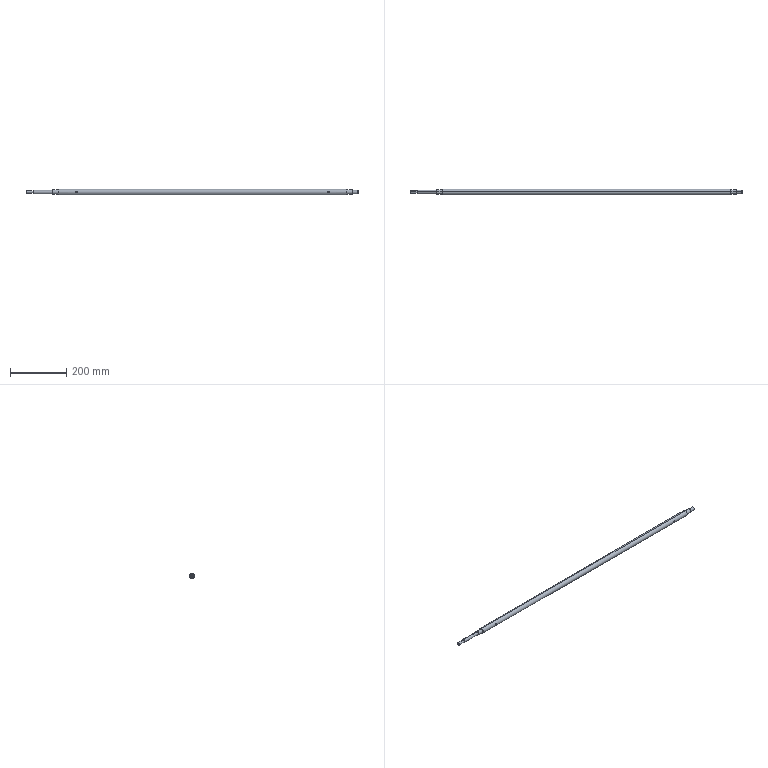Part | NX | features BREP 1 | 1 solid | 32 faces | box 1181 x 20 x 20 mm | volume 340275 mm3 | cylinder 18 | plane 10 | cone 4 | commonest cylinder face diameters 6 x4 12 x4 15 x4 4 x2 10 x2 20 x2
STEP:
#1=CARTESIAN_POINT('',(630.967,-9.539,-3.));
#2=VERTEX_POINT('',#1);
#3=CARTESIAN_POINT('',(630.967,-9.539,3.));
#4=VERTEX_POINT('',#3);
#5=CARTESIAN_POINT('',(630.967,-9.539,-3.));
#6=CARTESIAN_POINT('',(630.17,-9.539,-3.));
#7=CARTESIAN_POINT('',(628.623,-9.775,-2.35));
#8=CARTESIAN_POINT('',(627.639,-10.112,-0.004774));
#9=CARTESIAN_POINT('',(628.622,-9.775,2.351));
#10=CARTESIAN_POINT('',(630.17,-9.539,3.));
#11=CARTESIAN_POINT('',(630.967,-9.539,3.));
#12=B_SPLINE_CURVE_WITH_KNOTS('',3,(#5,#6,#7,#8,#9,#10,#11),.UNSPECIFIED.,.F.,.F.,(4,1,1,1,4),(0.,0.002358,0.004715,0.007073,0.009431),.UNSPECIFIED.);
#13=EDGE_CURVE('',#2,#4,#12,.T.);
#14=ORIENTED_EDGE('',*,*,#13,.F.);
#15=CARTESIAN_POINT('',(630.967,9.539,-3.));
#16=VERTEX_POINT('',#15);
#17=CARTESIAN_POINT('',(630.967,-10.,-3.));
#18=DIRECTION('',(0.,1.,0.));
#19=VECTOR('',#18,1000.);
#20=LINE('',#17,#19);
#21=EDGE_CURVE('',#2,#16,#20,.T.);
#22=ORIENTED_EDGE('',*,*,#21,.T.);
#23=CARTESIAN_POINT('',(630.967,9.539,3.));
#24=VERTEX_POINT('',#23);
#25=CARTESIAN_POINT('',(630.967,9.539,3.));
#26=CARTESIAN_POINT('',(630.17,9.539,3.));
#27=CARTESIAN_POINT('',(628.623,9.775,2.35));
#28=CARTESIAN_POINT('',(627.639,10.112,0.004774));
#29=CARTESIAN_POINT('',(628.622,9.775,-2.351));
#30=CARTESIAN_POINT('',(630.17,9.539,-3.));
#31=CARTESIAN_POINT('',(630.967,9.539,-3.));
#32=B_SPLINE_CURVE_WITH_KNOTS('',3,(#25,#26,#27,#28,#29,#30,#31),.UNSPECIFIED.,.F.,.F.,(4,1,1,1,4),(0.,0.002358,0.004715,0.007073,0.009431),.UNSPECIFIED.);
#33=EDGE_CURVE('',#24,#16,#32,.T.);
#34=ORIENTED_EDGE('',*,*,#33,.F.);
#35=CARTESIAN_POINT('',(630.967,-10.,3.));
#36=DIRECTION('',(0.,1.,0.));
#37=VECTOR('',#36,1000.);
#38=LINE('',#35,#37);
#39=EDGE_CURVE('',#4,#24,#38,.T.);
#40=ORIENTED_EDGE('',*,*,#39,.F.);
#41=EDGE_LOOP('',(#14,#22,#34,#40));
#42=FACE_BOUND('',#41,.T.);
#43=CARTESIAN_POINT('',(630.967,-10.,0.));
#44=DIRECTION('',(0.,1.,0.));
#45=DIRECTION('',(0.,0.,-1.));
#46=AXIS2_PLACEMENT_3D('',#43,#44,#45);
#47=CYLINDRICAL_SURFACE('',#46,3.);
#48=ADVANCED_FACE('',(#42),#47,.F.);
#49=CARTESIAN_POINT('',(-265.033,-9.539,-3.));
#50=VERTEX_POINT('',#49);
#51=CARTESIAN_POINT('',(-265.033,-9.539,3.));
#52=VERTEX_POINT('',#51);
#53=CARTESIAN_POINT('',(-265.033,-9.539,-3.));
#54=CARTESIAN_POINT('',(-265.83,-9.539,-3.));
#55=CARTESIAN_POINT('',(-267.377,-9.775,-2.35));
#56=CARTESIAN_POINT('',(-268.361,-10.112,-0.004774));
#57=CARTESIAN_POINT('',(-267.378,-9.775,2.351));
#58=CARTESIAN_POINT('',(-265.83,-9.539,3.));
#59=CARTESIAN_POINT('',(-265.033,-9.539,3.));
#60=B_SPLINE_CURVE_WITH_KNOTS('',3,(#53,#54,#55,#56,#57,#58,#59),.UNSPECIFIED.,.F.,.F.,(4,1,1,1,4),(0.,0.002358,0.004715,0.007073,0.009431),.UNSPECIFIED.);
#61=EDGE_CURVE('',#50,#52,#60,.T.);
#62=ORIENTED_EDGE('',*,*,#61,.F.);
#63=CARTESIAN_POINT('',(-265.033,9.539,-3.));
#64=VERTEX_POINT('',#63);
#65=CARTESIAN_POINT('',(-265.033,-10.,-3.));
#66=DIRECTION('',(0.,1.,0.));
#67=VECTOR('',#66,1000.);
#68=LINE('',#65,#67);
#69=EDGE_CURVE('',#50,#64,#68,.T.);
#70=ORIENTED_EDGE('',*,*,#69,.T.);
#71=CARTESIAN_POINT('',(-265.033,9.539,3.));
#72=VERTEX_POINT('',#71);
#73=CARTESIAN_POINT('',(-265.033,9.539,3.));
#74=CARTESIAN_POINT('',(-265.83,9.539,3.));
#75=CARTESIAN_POINT('',(-267.377,9.775,2.35));
#76=CARTESIAN_POINT('',(-268.361,10.112,0.004774));
#77=CARTESIAN_POINT('',(-267.378,9.775,-2.351));
#78=CARTESIAN_POINT('',(-265.83,9.539,-3.));
#79=CARTESIAN_POINT('',(-265.033,9.539,-3.));
#80=B_SPLINE_CURVE_WITH_KNOTS('',3,(#73,#74,#75,#76,#77,#78,#79),.UNSPECIFIED.,.F.,.F.,(4,1,1,1,4),(0.,0.002358,0.004715,0.007073,0.009431),.UNSPECIFIED.);
#81=EDGE_CURVE('',#72,#64,#80,.T.);
#82=ORIENTED_EDGE('',*,*,#81,.F.);
#83=CARTESIAN_POINT('',(-265.033,-10.,3.));
#84=DIRECTION('',(0.,1.,0.));
#85=VECTOR('',#84,1000.);
#86=LINE('',#83,#85);
#87=EDGE_CURVE('',#52,#72,#86,.T.);
#88=ORIENTED_EDGE('',*,*,#87,.F.);
#89=EDGE_LOOP('',(#62,#70,#82,#88));
#90=FACE_BOUND('',#89,.T.);
#91=CARTESIAN_POINT('',(-265.033,-10.,0.));
#92=DIRECTION('',(0.,1.,0.));
#93=DIRECTION('',(0.,0.,-1.));
#94=AXIS2_PLACEMENT_3D('',#91,#92,#93);
#95=CYLINDRICAL_SURFACE('',#94,3.);
#96=ADVANCED_FACE('',(#90),#95,.F.);
#97=CARTESIAN_POINT('',(735.967,0.,5.));
#98=VERTEX_POINT('',#97);
#99=CARTESIAN_POINT('',(735.967,0.,-5.));
#100=VERTEX_POINT('',#99);
#101=CARTESIAN_POINT('',(735.967,0.,0.));
#102=DIRECTION('',(-1.,0.,0.));
#103=DIRECTION('',(0.,0.,1.));
#104=AXIS2_PLACEMENT_3D('',#101,#102,#103);
#105=CIRCLE('',#104,5.);
#106=EDGE_CURVE('',#98,#100,#105,.T.);
#107=ORIENTED_EDGE('',*,*,#106,.T.);
#108=CARTESIAN_POINT('',(734.967,0.,-6.));
#109=VERTEX_POINT('',#108);
#110=CARTESIAN_POINT('',(735.967,0.,-5.));
#111=DIRECTION('',(-0.7071,0.,-0.7071));
#112=VECTOR('',#111,1000.);
#113=LINE('',#110,#112);
#114=EDGE_CURVE('',#100,#109,#113,.T.);
#115=ORIENTED_EDGE('',*,*,#114,.T.);
#116=CARTESIAN_POINT('',(734.967,0.,6.));
#117=VERTEX_POINT('',#116);
#118=CARTESIAN_POINT('',(734.967,0.,0.));
#119=DIRECTION('',(-1.,0.,0.));
#120=DIRECTION('',(0.,0.,1.));
#121=AXIS2_PLACEMENT_3D('',#118,#119,#120);
#122=CIRCLE('',#121,6.);
#123=EDGE_CURVE('',#117,#109,#122,.T.);
#124=ORIENTED_EDGE('',*,*,#123,.F.);
#125=CARTESIAN_POINT('',(735.967,0.,5.));
#126=DIRECTION('',(-0.7071,0.,0.7071));
#127=VECTOR('',#126,1000.);
#128=LINE('',#125,#127);
#129=EDGE_CURVE('',#98,#117,#128,.T.);
#130=ORIENTED_EDGE('',*,*,#129,.F.);
#131=EDGE_LOOP('',(#107,#115,#124,#130));
#132=FACE_BOUND('',#131,.T.);
#133=CARTESIAN_POINT('',(735.967,0.,0.));
#134=DIRECTION('',(-1.,0.,0.));
#135=DIRECTION('',(0.,0.,-1.));
#136=AXIS2_PLACEMENT_3D('',#133,#134,#135);
#137=CONICAL_SURFACE('',#136,5.,0.7854);
#138=ADVANCED_FACE('',(#132),#137,.T.);
#139=ORIENTED_EDGE('',*,*,#123,.T.);
#140=CARTESIAN_POINT('',(715.967,0.,-6.));
#141=VERTEX_POINT('',#140);
#142=CARTESIAN_POINT('',(-445.033,0.,-6.));
#143=DIRECTION('',(-1.,0.,0.));
#144=VECTOR('',#143,1000.);
#145=LINE('',#142,#144);
#146=EDGE_CURVE('',#109,#141,#145,.T.);
#147=ORIENTED_EDGE('',*,*,#146,.T.);
#148=CARTESIAN_POINT('',(715.967,0.,6.));
#149=VERTEX_POINT('',#148);
#150=CARTESIAN_POINT('',(715.967,0.,0.));
#151=DIRECTION('',(-1.,0.,0.));
#152=DIRECTION('',(0.,0.,1.));
#153=AXIS2_PLACEMENT_3D('',#150,#151,#152);
#154=CIRCLE('',#153,6.);
#155=EDGE_CURVE('',#149,#141,#154,.T.);
#156=ORIENTED_EDGE('',*,*,#155,.F.);
#157=CARTESIAN_POINT('',(-445.033,0.,6.));
#158=DIRECTION('',(-1.,0.,0.));
#159=VECTOR('',#158,1000.);
#160=LINE('',#157,#159);
#161=EDGE_CURVE('',#117,#149,#160,.T.);
#162=ORIENTED_EDGE('',*,*,#161,.F.);
#163=EDGE_LOOP('',(#139,#147,#156,#162));
#164=FACE_BOUND('',#163,.T.);
#165=CARTESIAN_POINT('',(-445.033,0.,0.));
#166=DIRECTION('',(-1.,0.,0.));
#167=DIRECTION('',(0.,0.,-1.));
#168=AXIS2_PLACEMENT_3D('',#165,#166,#167);
#169=CYLINDRICAL_SURFACE('',#168,6.);
#170=ADVANCED_FACE('',(#164),#169,.T.);
#171=CARTESIAN_POINT('',(715.967,0.,7.5));
#172=VERTEX_POINT('',#171);
#173=CARTESIAN_POINT('',(715.967,0.,-7.5));
#174=VERTEX_POINT('',#173);
#175=CARTESIAN_POINT('',(715.967,0.,0.));
#176=DIRECTION('',(-1.,0.,0.));
#177=DIRECTION('',(0.,0.,1.));
#178=AXIS2_PLACEMENT_3D('',#175,#176,#177);
#179=CIRCLE('',#178,7.5);
#180=EDGE_CURVE('',#172,#174,#179,.T.);
#181=ORIENTED_EDGE('',*,*,#180,.T.);
#182=CARTESIAN_POINT('',(695.967,0.,-7.5));
#183=VERTEX_POINT('',#182);
#184=CARTESIAN_POINT('',(-445.033,0.,-7.5));
#185=DIRECTION('',(-1.,0.,0.));
#186=VECTOR('',#185,1000.);
#187=LINE('',#184,#186);
#188=EDGE_CURVE('',#174,#183,#187,.T.);
#189=ORIENTED_EDGE('',*,*,#188,.T.);
#190=CARTESIAN_POINT('',(695.967,0.,7.5));
#191=VERTEX_POINT('',#190);
#192=CARTESIAN_POINT('',(695.967,0.,0.));
#193=DIRECTION('',(-1.,0.,0.));
#194=DIRECTION('',(0.,0.,1.));
#195=AXIS2_PLACEMENT_3D('',#192,#193,#194);
#196=CIRCLE('',#195,7.5);
#197=EDGE_CURVE('',#191,#183,#196,.T.);
#198=ORIENTED_EDGE('',*,*,#197,.F.);
#199=CARTESIAN_POINT('',(-445.033,0.,7.5));
#200=DIRECTION('',(-1.,0.,0.));
#201=VECTOR('',#200,1000.);
#202=LINE('',#199,#201);
#203=EDGE_CURVE('',#172,#191,#202,.T.);
#204=ORIENTED_EDGE('',*,*,#203,.F.);
#205=EDGE_LOOP('',(#181,#189,#198,#204));
#206=FACE_BOUND('',#205,.T.);
#207=CARTESIAN_POINT('',(-445.033,0.,0.));
#208=DIRECTION('',(-1.,0.,0.));
#209=DIRECTION('',(0.,0.,-1.));
#210=AXIS2_PLACEMENT_3D('',#207,#208,#209);
#211=CYLINDRICAL_SURFACE('',#210,7.5);
#212=ADVANCED_FACE('',(#206),#211,.T.);
#213=CARTESIAN_POINT('',(695.967,0.,10.));
#214=VERTEX_POINT('',#213);
#215=CARTESIAN_POINT('',(695.967,0.,-10.));
#216=VERTEX_POINT('',#215);
#217=CARTESIAN_POINT('',(695.967,0.,0.));
#218=DIRECTION('',(-1.,0.,0.));
#219=DIRECTION('',(0.,0.,1.));
#220=AXIS2_PLACEMENT_3D('',#217,#218,#219);
#221=CIRCLE('',#220,10.);
#222=EDGE_CURVE('',#214,#216,#221,.T.);
#223=ORIENTED_EDGE('',*,*,#222,.T.);
#224=CARTESIAN_POINT('',(-330.033,0.,-10.));
#225=VERTEX_POINT('',#224);
#226=CARTESIAN_POINT('',(-445.033,0.,-10.));
#227=DIRECTION('',(-1.,0.,0.));
#228=VECTOR('',#227,1000.);
#229=LINE('',#226,#228);
#230=EDGE_CURVE('',#216,#225,#229,.T.);
#231=ORIENTED_EDGE('',*,*,#230,.T.);
#232=CARTESIAN_POINT('',(-330.033,0.,10.));
#233=VERTEX_POINT('',#232);
#234=CARTESIAN_POINT('',(-330.033,0.,0.));
#235=DIRECTION('',(-1.,0.,0.));
#236=DIRECTION('',(0.,0.,1.));
#237=AXIS2_PLACEMENT_3D('',#234,#235,#236);
#238=CIRCLE('',#237,10.);
#239=EDGE_CURVE('',#233,#225,#238,.T.);
#240=ORIENTED_EDGE('',*,*,#239,.F.);
#241=CARTESIAN_POINT('',(-445.033,0.,10.));
#242=DIRECTION('',(-1.,0.,0.));
#243=VECTOR('',#242,1000.);
#244=LINE('',#241,#243);
#245=EDGE_CURVE('',#214,#233,#244,.T.);
#246=ORIENTED_EDGE('',*,*,#245,.F.);
#247=EDGE_LOOP('',(#223,#231,#240,#246));
#248=FACE_BOUND('',#247,.T.);
#249=ORIENTED_EDGE('',*,*,#81,.T.);
#250=CARTESIAN_POINT('',(-265.033,9.539,-3.));
#251=CARTESIAN_POINT('',(-264.235,9.539,-3.));
#252=CARTESIAN_POINT('',(-262.689,9.775,-2.35));
#253=CARTESIAN_POINT('',(-261.705,10.112,-0.004774));
#254=CARTESIAN_POINT('',(-262.688,9.775,2.351));
#255=CARTESIAN_POINT('',(-264.235,9.539,3.));
#256=CARTESIAN_POINT('',(-265.033,9.539,3.));
#257=B_SPLINE_CURVE_WITH_KNOTS('',3,(#250,#251,#252,#253,#254,#255,#256),.UNSPECIFIED.,.F.,.F.,(4,1,1,1,4),(0.,0.002358,0.004715,0.007073,0.009431),.UNSPECIFIED.);
#258=EDGE_CURVE('',#64,#72,#257,.T.);
#259=ORIENTED_EDGE('',*,*,#258,.T.);
#260=EDGE_LOOP('',(#249,#259));
#261=FACE_BOUND('',#260,.T.);
#262=ORIENTED_EDGE('',*,*,#33,.T.);
#263=CARTESIAN_POINT('',(630.967,9.539,-3.));
#264=CARTESIAN_POINT('',(631.765,9.539,-3.));
#265=CARTESIAN_POINT('',(633.311,9.775,-2.35));
#266=CARTESIAN_POINT('',(634.295,10.112,-0.004774));
#267=CARTESIAN_POINT('',(633.312,9.775,2.351));
#268=CARTESIAN_POINT('',(631.765,9.539,3.));
#269=CARTESIAN_POINT('',(630.967,9.539,3.));
#270=B_SPLINE_CURVE_WITH_KNOTS('',3,(#263,#264,#265,#266,#267,#268,#269),.UNSPECIFIED.,.F.,.F.,(4,1,1,1,4),(0.,0.002358,0.004715,0.007073,0.009431),.UNSPECIFIED.);
#271=EDGE_CURVE('',#16,#24,#270,.T.);
#272=ORIENTED_EDGE('',*,*,#271,.T.);
#273=EDGE_LOOP('',(#262,#272));
#274=FACE_BOUND('',#273,.T.);
#275=CARTESIAN_POINT('',(-445.033,0.,0.));
#276=DIRECTION('',(-1.,0.,0.));
#277=DIRECTION('',(0.,0.,-1.));
#278=AXIS2_PLACEMENT_3D('',#275,#276,#277);
#279=CYLINDRICAL_SURFACE('',#278,10.);
#280=ADVANCED_FACE('',(#248,#261,#274),#279,.T.);
#281=CARTESIAN_POINT('',(-330.033,0.,7.5));
#282=VERTEX_POINT('',#281);
#283=CARTESIAN_POINT('',(-330.033,0.,-7.5));
#284=VERTEX_POINT('',#283);
#285=CARTESIAN_POINT('',(-330.033,0.,0.));
#286=DIRECTION('',(-1.,0.,0.));
#287=DIRECTION('',(0.,0.,1.));
#288=AXIS2_PLACEMENT_3D('',#285,#286,#287);
#289=CIRCLE('',#288,7.5);
#290=EDGE_CURVE('',#282,#284,#289,.T.);
#291=ORIENTED_EDGE('',*,*,#290,.T.);
#292=CARTESIAN_POINT('',(-350.033,0.,-7.5));
#293=VERTEX_POINT('',#292);
#294=CARTESIAN_POINT('',(-445.033,0.,-7.5));
#295=DIRECTION('',(-1.,0.,0.));
#296=VECTOR('',#295,1000.);
#297=LINE('',#294,#296);
#298=EDGE_CURVE('',#284,#293,#297,.T.);
#299=ORIENTED_EDGE('',*,*,#298,.T.);
#300=CARTESIAN_POINT('',(-350.033,0.,7.5));
#301=VERTEX_POINT('',#300);
#302=CARTESIAN_POINT('',(-350.033,0.,0.));
#303=DIRECTION('',(-1.,0.,0.));
#304=DIRECTION('',(0.,0.,1.));
#305=AXIS2_PLACEMENT_3D('',#302,#303,#304);
#306=CIRCLE('',#305,7.5);
#307=EDGE_CURVE('',#301,#293,#306,.T.);
#308=ORIENTED_EDGE('',*,*,#307,.F.);
#309=CARTESIAN_POINT('',(-445.033,0.,7.5));
#310=DIRECTION('',(-1.,0.,0.));
#311=VECTOR('',#310,1000.);
#312=LINE('',#309,#311);
#313=EDGE_CURVE('',#282,#301,#312,.T.);
#314=ORIENTED_EDGE('',*,*,#313,.F.);
#315=EDGE_LOOP('',(#291,#299,#308,#314));
#316=FACE_BOUND('',#315,.T.);
#317=CARTESIAN_POINT('',(-445.033,0.,0.));
#318=DIRECTION('',(-1.,0.,0.));
#319=DIRECTION('',(0.,0.,-1.));
#320=AXIS2_PLACEMENT_3D('',#317,#318,#319);
#321=CYLINDRICAL_SURFACE('',#320,7.5);
#322=ADVANCED_FACE('',(#316),#321,.T.);
#323=CARTESIAN_POINT('',(-350.033,0.,6.));
#324=VERTEX_POINT('',#323);
#325=CARTESIAN_POINT('',(-350.033,0.,-6.));
#326=VERTEX_POINT('',#325);
#327=CARTESIAN_POINT('',(-350.033,0.,0.));
#328=DIRECTION('',(-1.,0.,0.));
#329=DIRECTION('',(0.,0.,1.));
#330=AXIS2_PLACEMENT_3D('',#327,#328,#329);
#331=CIRCLE('',#330,6.);
#332=EDGE_CURVE('',#324,#326,#331,.T.);
#333=ORIENTED_EDGE('',*,*,#332,.T.);
#334=CARTESIAN_POINT('',(-420.033,0.,-6.));
#335=VERTEX_POINT('',#334);
#336=CARTESIAN_POINT('',(-445.033,0.,-6.));
#337=DIRECTION('',(-1.,0.,0.));
#338=VECTOR('',#337,1000.);
#339=LINE('',#336,#338);
#340=EDGE_CURVE('',#326,#335,#339,.T.);
#341=ORIENTED_EDGE('',*,*,#340,.T.);
#342=CARTESIAN_POINT('',(-420.033,0.,6.));
#343=VERTEX_POINT('',#342);
#344=CARTESIAN_POINT('',(-420.033,0.,0.));
#345=DIRECTION('',(-1.,0.,0.));
#346=DIRECTION('',(0.,0.,1.));
#347=AXIS2_PLACEMENT_3D('',#344,#345,#346);
#348=CIRCLE('',#347,6.);
#349=EDGE_CURVE('',#343,#335,#348,.T.);
#350=ORIENTED_EDGE('',*,*,#349,.F.);
#351=CARTESIAN_POINT('',(-445.033,0.,6.));
#352=DIRECTION('',(-1.,0.,0.));
#353=VECTOR('',#352,1000.);
#354=LINE('',#351,#353);
#355=EDGE_CURVE('',#324,#343,#354,.T.);
#356=ORIENTED_EDGE('',*,*,#355,.F.);
#357=EDGE_LOOP('',(#333,#341,#350,#356));
#358=FACE_BOUND('',#357,.T.);
#359=CARTESIAN_POINT('',(-445.033,0.,0.));
#360=DIRECTION('',(-1.,0.,0.));
#361=DIRECTION('',(0.,0.,-1.));
#362=AXIS2_PLACEMENT_3D('',#359,#360,#361);
#363=CYLINDRICAL_SURFACE('',#362,6.);
#364=ADVANCED_FACE('',(#358),#363,.T.);
#365=CARTESIAN_POINT('',(-420.033,0.,5.));
#366=VERTEX_POINT('',#365);
#367=CARTESIAN_POINT('',(-420.033,0.,-5.));
#368=VERTEX_POINT('',#367);
#369=CARTESIAN_POINT('',(-420.033,0.,0.));
#370=DIRECTION('',(-1.,0.,0.));
#371=DIRECTION('',(0.,0.,1.));
#372=AXIS2_PLACEMENT_3D('',#369,#370,#371);
#373=CIRCLE('',#372,5.);
#374=EDGE_CURVE('',#366,#368,#373,.T.);
#375=ORIENTED_EDGE('',*,*,#374,.T.);
#376=CARTESIAN_POINT('',(-444.033,0.,-5.));
#377=VERTEX_POINT('',#376);
#378=CARTESIAN_POINT('',(-445.033,0.,-5.));
#379=DIRECTION('',(-1.,0.,0.));
#380=VECTOR('',#379,1000.);
#381=LINE('',#378,#380);
#382=EDGE_CURVE('',#368,#377,#381,.T.);
#383=ORIENTED_EDGE('',*,*,#382,.T.);
#384=CARTESIAN_POINT('',(-444.033,0.,5.));
#385=VERTEX_POINT('',#384);
#386=CARTESIAN_POINT('',(-444.033,0.,0.));
#387=DIRECTION('',(-1.,0.,0.));
#388=DIRECTION('',(0.,0.,1.));
#389=AXIS2_PLACEMENT_3D('',#386,#387,#388);
#390=CIRCLE('',#389,5.);
#391=EDGE_CURVE('',#385,#377,#390,.T.);
#392=ORIENTED_EDGE('',*,*,#391,.F.);
#393=CARTESIAN_POINT('',(-445.033,0.,5.));
#394=DIRECTION('',(-1.,0.,0.));
#395=VECTOR('',#394,1000.);
#396=LINE('',#393,#395);
#397=EDGE_CURVE('',#366,#385,#396,.T.);
#398=ORIENTED_EDGE('',*,*,#397,.F.);
#399=EDGE_LOOP('',(#375,#383,#392,#398));
#400=FACE_BOUND('',#399,.T.);
#401=CARTESIAN_POINT('',(-437.033,4.583,-2.));
#402=VERTEX_POINT('',#401);
#403=CARTESIAN_POINT('',(-425.033,4.583,-2.));
#404=VERTEX_POINT('',#403);
#405=CARTESIAN_POINT('',(-445.033,4.583,-2.));
#406=DIRECTION('',(1.,0.,0.));
#407=VECTOR('',#406,1000.);
#408=LINE('',#405,#407);
#409=EDGE_CURVE('',#402,#404,#408,.T.);
#410=ORIENTED_EDGE('',*,*,#409,.T.);
#411=CARTESIAN_POINT('',(-425.033,4.583,2.));
#412=VERTEX_POINT('',#411);
#413=CARTESIAN_POINT('',(-425.033,4.583,-2.));
#414=CARTESIAN_POINT('',(-424.498,4.583,-2.));
#415=CARTESIAN_POINT('',(-423.472,4.8,-1.567));
#416=CARTESIAN_POINT('',(-422.813,5.1,-0.004067));
#417=CARTESIAN_POINT('',(-423.472,4.8,1.568));
#418=CARTESIAN_POINT('',(-424.498,4.583,2.));
#419=CARTESIAN_POINT('',(-425.033,4.583,2.));
#420=B_SPLINE_CURVE_WITH_KNOTS('',3,(#413,#414,#415,#416,#417,#418,#419),.UNSPECIFIED.,.F.,.F.,(4,1,1,1,4),(0.,0.001579,0.003158,0.004737,0.006317),.UNSPECIFIED.);
#421=EDGE_CURVE('',#404,#412,#420,.T.);
#422=ORIENTED_EDGE('',*,*,#421,.T.);
#423=CARTESIAN_POINT('',(-437.033,4.583,2.));
#424=VERTEX_POINT('',#423);
#425=CARTESIAN_POINT('',(-445.033,4.583,2.));
#426=DIRECTION('',(-1.,0.,0.));
#427=VECTOR('',#426,1000.);
#428=LINE('',#425,#427);
#429=EDGE_CURVE('',#412,#424,#428,.T.);
#430=ORIENTED_EDGE('',*,*,#429,.T.);
#431=CARTESIAN_POINT('',(-437.033,4.583,2.));
#432=CARTESIAN_POINT('',(-437.567,4.583,2.));
#433=CARTESIAN_POINT('',(-438.593,4.8,1.567));
#434=CARTESIAN_POINT('',(-439.252,5.1,0.004067));
#435=CARTESIAN_POINT('',(-438.594,4.8,-1.568));
#436=CARTESIAN_POINT('',(-437.567,4.583,-2.));
#437=CARTESIAN_POINT('',(-437.033,4.583,-2.));
#438=B_SPLINE_CURVE_WITH_KNOTS('',3,(#431,#432,#433,#434,#435,#436,#437),.UNSPECIFIED.,.F.,.F.,(4,1,1,1,4),(0.,0.001579,0.003158,0.004737,0.006317),.UNSPECIFIED.);
#439=EDGE_CURVE('',#424,#402,#438,.T.);
#440=ORIENTED_EDGE('',*,*,#439,.T.);
#441=EDGE_LOOP('',(#410,#422,#430,#440));
#442=FACE_BOUND('',#441,.T.);
#443=CARTESIAN_POINT('',(-445.033,0.,0.));
#444=DIRECTION('',(-1.,0.,0.));
#445=DIRECTION('',(0.,0.,-1.));
#446=AXIS2_PLACEMENT_3D('',#443,#444,#445);
#447=CYLINDRICAL_SURFACE('',#446,5.);
#448=ADVANCED_FACE('',(#400,#442),#447,.T.);
#449=CARTESIAN_POINT('',(-445.033,0.,4.));
#450=VERTEX_POINT('',#449);
#451=CARTESIAN_POINT('',(-445.033,0.,-4.));
#452=VERTEX_POINT('',#451);
#453=CARTESIAN_POINT('',(-445.033,0.,0.));
#454=DIRECTION('',(-1.,0.,0.));
#455=DIRECTION('',(0.,0.,1.));
#456=AXIS2_PLACEMENT_3D('',#453,#454,#455);
#457=CIRCLE('',#456,4.);
#458=EDGE_CURVE('',#450,#452,#457,.T.);
#459=ORIENTED_EDGE('',*,*,#458,.F.);
#460=CARTESIAN_POINT('',(-444.033,0.,5.));
#461=DIRECTION('',(0.7071,0.,0.7071));
#462=VECTOR('',#461,1000.);
#463=LINE('',#460,#462);
#464=EDGE_CURVE('',#385,#450,#463,.F.);
#465=ORIENTED_EDGE('',*,*,#464,.F.);
#466=ORIENTED_EDGE('',*,*,#391,.T.);
#467=CARTESIAN_POINT('',(-444.033,0.,-5.));
#468=DIRECTION('',(0.7071,0.,-0.7071));
#469=VECTOR('',#468,1000.);
#470=LINE('',#467,#469);
#471=EDGE_CURVE('',#377,#452,#470,.F.);
#472=ORIENTED_EDGE('',*,*,#471,.T.);
#473=EDGE_LOOP('',(#459,#465,#466,#472));
#474=FACE_BOUND('',#473,.T.);
#475=CARTESIAN_POINT('',(-444.033,0.,0.));
#476=DIRECTION('',(1.,0.,0.));
#477=DIRECTION('',(0.,0.,1.));
#478=AXIS2_PLACEMENT_3D('',#475,#476,#477);
#479=CONICAL_SURFACE('',#478,5.,0.7854);
#480=ADVANCED_FACE('',(#474),#479,.T.);
#481=ORIENTED_EDGE('',*,*,#464,.T.);
#482=CARTESIAN_POINT('',(-445.033,0.,0.));
#483=DIRECTION('',(-1.,0.,0.));
#484=DIRECTION('',(0.,0.,1.));
#485=AXIS2_PLACEMENT_3D('',#482,#483,#484);
#486=CIRCLE('',#485,4.);
#487=EDGE_CURVE('',#452,#450,#486,.T.);
#488=ORIENTED_EDGE('',*,*,#487,.F.);
#489=ORIENTED_EDGE('',*,*,#471,.F.);
#490=CARTESIAN_POINT('',(-444.033,0.,0.));
#491=DIRECTION('',(-1.,0.,0.));
#492=DIRECTION('',(0.,0.,1.));
#493=AXIS2_PLACEMENT_3D('',#490,#491,#492);
#494=CIRCLE('',#493,5.);
#495=EDGE_CURVE('',#377,#385,#494,.T.);
#496=ORIENTED_EDGE('',*,*,#495,.T.);
#497=EDGE_LOOP('',(#481,#488,#489,#496));
#498=FACE_BOUND('',#497,.T.);
#499=CARTESIAN_POINT('',(-444.033,0.,0.));
#500=DIRECTION('',(1.,0.,0.));
#501=DIRECTION('',(0.,0.,1.));
#502=AXIS2_PLACEMENT_3D('',#499,#500,#501);
#503=CONICAL_SURFACE('',#502,5.,0.7854);
#504=ADVANCED_FACE('',(#498),#503,.T.);
#505=ORIENTED_EDGE('',*,*,#382,.F.);
#506=CARTESIAN_POINT('',(-420.033,0.,0.));
#507=DIRECTION('',(-1.,0.,0.));
#508=DIRECTION('',(0.,0.,1.));
#509=AXIS2_PLACEMENT_3D('',#506,#507,#508);
#510=CIRCLE('',#509,5.);
#511=EDGE_CURVE('',#368,#366,#510,.T.);
#512=ORIENTED_EDGE('',*,*,#511,.T.);
#513=ORIENTED_EDGE('',*,*,#397,.T.);
#514=ORIENTED_EDGE('',*,*,#495,.F.);
#515=EDGE_LOOP('',(#505,#512,#513,#514));
#516=FACE_BOUND('',#515,.T.);
#517=CARTESIAN_POINT('',(-445.033,0.,0.));
#518=DIRECTION('',(-1.,0.,0.));
#519=DIRECTION('',(0.,0.,-1.));
#520=AXIS2_PLACEMENT_3D('',#517,#518,#519);
#521=CYLINDRICAL_SURFACE('',#520,5.);
#522=ADVANCED_FACE('',(#516),#521,.T.);
#523=ORIENTED_EDGE('',*,*,#349,.T.);
#524=CARTESIAN_POINT('',(-420.033,0.,0.));
#525=DIRECTION('',(-1.,0.,0.));
#526=DIRECTION('',(0.,0.,1.));
#527=AXIS2_PLACEMENT_3D('',#524,#525,#526);
#528=CIRCLE('',#527,6.);
#529=EDGE_CURVE('',#335,#343,#528,.T.);
#530=ORIENTED_EDGE('',*,*,#529,.T.);
#531=EDGE_LOOP('',(#523,#530));
#532=FACE_BOUND('',#531,.T.);
#533=ORIENTED_EDGE('',*,*,#374,.F.);
#534=ORIENTED_EDGE('',*,*,#511,.F.);
#535=EDGE_LOOP('',(#533,#534));
#536=FACE_BOUND('',#535,.T.);
#537=CARTESIAN_POINT('',(-420.033,5.,0.));
#538=DIRECTION('',(1.,0.,0.));
#539=DIRECTION('',(0.,0.,1.));
#540=AXIS2_PLACEMENT_3D('',#537,#538,#539);
#541=PLANE('',#540);
#542=ADVANCED_FACE('',(#532,#536),#541,.F.);
#543=ORIENTED_EDGE('',*,*,#340,.F.);
#544=CARTESIAN_POINT('',(-350.033,0.,0.));
#545=DIRECTION('',(-1.,0.,0.));
#546=DIRECTION('',(0.,0.,1.));
#547=AXIS2_PLACEMENT_3D('',#544,#545,#546);
#548=CIRCLE('',#547,6.);
#549=EDGE_CURVE('',#326,#324,#548,.T.);
#550=ORIENTED_EDGE('',*,*,#549,.T.);
#551=ORIENTED_EDGE('',*,*,#355,.T.);
#552=ORIENTED_EDGE('',*,*,#529,.F.);
#553=EDGE_LOOP('',(#543,#550,#551,#552));
#554=FACE_BOUND('',#553,.T.);
#555=CARTESIAN_POINT('',(-445.033,0.,0.));
#556=DIRECTION('',(-1.,0.,0.));
#557=DIRECTION('',(0.,0.,-1.));
#558=AXIS2_PLACEMENT_3D('',#555,#556,#557);
#559=CYLINDRICAL_SURFACE('',#558,6.);
#560=ADVANCED_FACE('',(#554),#559,.T.);
#561=ORIENTED_EDGE('',*,*,#307,.T.);
#562=CARTESIAN_POINT('',(-350.033,0.,0.));
#563=DIRECTION('',(-1.,0.,0.));
#564=DIRECTION('',(0.,0.,1.));
#565=AXIS2_PLACEMENT_3D('',#562,#563,#564);
#566=CIRCLE('',#565,7.5);
#567=EDGE_CURVE('',#293,#301,#566,.T.);
#568=ORIENTED_EDGE('',*,*,#567,.T.);
#569=EDGE_LOOP('',(#561,#568));
#570=FACE_BOUND('',#569,.T.);
#571=ORIENTED_EDGE('',*,*,#332,.F.);
#572=ORIENTED_EDGE('',*,*,#549,.F.);
#573=EDGE_LOOP('',(#571,#572));
#574=FACE_BOUND('',#573,.T.);
#575=CARTESIAN_POINT('',(-350.033,6.,0.));
#576=DIRECTION('',(1.,0.,0.));
#577=DIRECTION('',(0.,0.,1.));
#578=AXIS2_PLACEMENT_3D('',#575,#576,#577);
#579=PLANE('',#578);
#580=ADVANCED_FACE('',(#570,#574),#579,.F.);
#581=ORIENTED_EDGE('',*,*,#298,.F.);
#582=CARTESIAN_POINT('',(-330.033,0.,0.));
#583=DIRECTION('',(-1.,0.,0.));
#584=DIRECTION('',(0.,0.,1.));
#585=AXIS2_PLACEMENT_3D('',#582,#583,#584);
#586=CIRCLE('',#585,7.5);
#587=EDGE_CURVE('',#284,#282,#586,.T.);
#588=ORIENTED_EDGE('',*,*,#587,.T.);
#589=ORIENTED_EDGE('',*,*,#313,.T.);
#590=ORIENTED_EDGE('',*,*,#567,.F.);
#591=EDGE_LOOP('',(#581,#588,#589,#590));
#592=FACE_BOUND('',#591,.T.);
#593=CARTESIAN_POINT('',(-445.033,0.,0.));
#594=DIRECTION('',(-1.,0.,0.));
#595=DIRECTION('',(0.,0.,-1.));
#596=AXIS2_PLACEMENT_3D('',#593,#594,#595);
#597=CYLINDRICAL_SURFACE('',#596,7.5);
#598=ADVANCED_FACE('',(#592),#597,.T.);
#599=ORIENTED_EDGE('',*,*,#239,.T.);
#600=CARTESIAN_POINT('',(-330.033,0.,0.));
#601=DIRECTION('',(-1.,0.,0.));
#602=DIRECTION('',(0.,0.,1.));
#603=AXIS2_PLACEMENT_3D('',#600,#601,#602);
#604=CIRCLE('',#603,10.);
#605=EDGE_CURVE('',#225,#233,#604,.T.);
#606=ORIENTED_EDGE('',*,*,#605,.T.);
#607=EDGE_LOOP('',(#599,#606));
#608=FACE_BOUND('',#607,.T.);
#609=ORIENTED_EDGE('',*,*,#290,.F.);
#610=ORIENTED_EDGE('',*,*,#587,.F.);
#611=EDGE_LOOP('',(#609,#610));
#612=FACE_BOUND('',#611,.T.);
#613=CARTESIAN_POINT('',(-330.033,7.5,0.));
#614=DIRECTION('',(1.,0.,0.));
#615=DIRECTION('',(0.,0.,1.));
#616=AXIS2_PLACEMENT_3D('',#613,#614,#615);
#617=PLANE('',#616);
#618=ADVANCED_FACE('',(#608,#612),#617,.F.);
#619=ORIENTED_EDGE('',*,*,#230,.F.);
#620=CARTESIAN_POINT('',(695.967,0.,0.));
#621=DIRECTION('',(-1.,0.,0.));
#622=DIRECTION('',(0.,0.,1.));
#623=AXIS2_PLACEMENT_3D('',#620,#621,#622);
#624=CIRCLE('',#623,10.);
#625=EDGE_CURVE('',#216,#214,#624,.T.);
#626=ORIENTED_EDGE('',*,*,#625,.T.);
#627=ORIENTED_EDGE('',*,*,#245,.T.);
#628=ORIENTED_EDGE('',*,*,#605,.F.);
#629=EDGE_LOOP('',(#619,#626,#627,#628));
#630=FACE_BOUND('',#629,.T.);
#631=CARTESIAN_POINT('',(630.967,-9.539,3.));
#632=CARTESIAN_POINT('',(631.765,-9.539,3.));
#633=CARTESIAN_POINT('',(633.311,-9.775,2.35));
#634=CARTESIAN_POINT('',(634.295,-10.112,0.004774));
#635=CARTESIAN_POINT('',(633.312,-9.775,-2.351));
#636=CARTESIAN_POINT('',(631.765,-9.539,-3.));
#637=CARTESIAN_POINT('',(630.967,-9.539,-3.));
#638=B_SPLINE_CURVE_WITH_KNOTS('',3,(#631,#632,#633,#634,#635,#636,#637),.UNSPECIFIED.,.F.,.F.,(4,1,1,1,4),(0.,0.002358,0.004715,0.007073,0.009431),.UNSPECIFIED.);
#639=EDGE_CURVE('',#4,#2,#638,.T.);
#640=ORIENTED_EDGE('',*,*,#639,.T.);
#641=ORIENTED_EDGE('',*,*,#13,.T.);
#642=EDGE_LOOP('',(#640,#641));
#643=FACE_BOUND('',#642,.T.);
#644=CARTESIAN_POINT('',(-265.033,-9.539,3.));
#645=CARTESIAN_POINT('',(-264.235,-9.539,3.));
#646=CARTESIAN_POINT('',(-262.689,-9.775,2.35));
#647=CARTESIAN_POINT('',(-261.705,-10.112,0.004774));
#648=CARTESIAN_POINT('',(-262.688,-9.775,-2.351));
#649=CARTESIAN_POINT('',(-264.235,-9.539,-3.));
#650=CARTESIAN_POINT('',(-265.033,-9.539,-3.));
#651=B_SPLINE_CURVE_WITH_KNOTS('',3,(#644,#645,#646,#647,#648,#649,#650),.UNSPECIFIED.,.F.,.F.,(4,1,1,1,4),(0.,0.002358,0.004715,0.007073,0.009431),.UNSPECIFIED.);
#652=EDGE_CURVE('',#52,#50,#651,.T.);
#653=ORIENTED_EDGE('',*,*,#652,.T.);
#654=ORIENTED_EDGE('',*,*,#61,.T.);
#655=EDGE_LOOP('',(#653,#654));
#656=FACE_BOUND('',#655,.T.);
#657=CARTESIAN_POINT('',(-445.033,0.,0.));
#658=DIRECTION('',(-1.,0.,0.));
#659=DIRECTION('',(0.,0.,-1.));
#660=AXIS2_PLACEMENT_3D('',#657,#658,#659);
#661=CYLINDRICAL_SURFACE('',#660,10.);
#662=ADVANCED_FACE('',(#630,#643,#656),#661,.T.);
#663=ORIENTED_EDGE('',*,*,#222,.F.);
#664=ORIENTED_EDGE('',*,*,#625,.F.);
#665=EDGE_LOOP('',(#663,#664));
#666=FACE_BOUND('',#665,.T.);
#667=ORIENTED_EDGE('',*,*,#197,.T.);
#668=CARTESIAN_POINT('',(695.967,0.,0.));
#669=DIRECTION('',(-1.,0.,0.));
#670=DIRECTION('',(0.,0.,1.));
#671=AXIS2_PLACEMENT_3D('',#668,#669,#670);
#672=CIRCLE('',#671,7.5);
#673=EDGE_CURVE('',#183,#191,#672,.T.);
#674=ORIENTED_EDGE('',*,*,#673,.T.);
#675=EDGE_LOOP('',(#667,#674));
#676=FACE_BOUND('',#675,.T.);
#677=CARTESIAN_POINT('',(695.967,10.,0.));
#678=DIRECTION('',(-1.,0.,0.));
#679=DIRECTION('',(0.,-1.,0.));
#680=AXIS2_PLACEMENT_3D('',#677,#678,#679);
#681=PLANE('',#680);
#682=ADVANCED_FACE('',(#666,#676),#681,.F.);
#683=ORIENTED_EDGE('',*,*,#188,.F.);
#684=CARTESIAN_POINT('',(715.967,0.,0.));
#685=DIRECTION('',(-1.,0.,0.));
#686=DIRECTION('',(0.,0.,1.));
#687=AXIS2_PLACEMENT_3D('',#684,#685,#686);
#688=CIRCLE('',#687,7.5);
#689=EDGE_CURVE('',#174,#172,#688,.T.);
#690=ORIENTED_EDGE('',*,*,#689,.T.);
#691=ORIENTED_EDGE('',*,*,#203,.T.);
#692=ORIENTED_EDGE('',*,*,#673,.F.);
#693=EDGE_LOOP('',(#683,#690,#691,#692));
#694=FACE_BOUND('',#693,.T.);
#695=CARTESIAN_POINT('',(-445.033,0.,0.));
#696=DIRECTION('',(-1.,0.,0.));
#697=DIRECTION('',(0.,0.,-1.));
#698=AXIS2_PLACEMENT_3D('',#695,#696,#697);
#699=CYLINDRICAL_SURFACE('',#698,7.5);
#700=ADVANCED_FACE('',(#694),#699,.T.);
#701=ORIENTED_EDGE('',*,*,#180,.F.);
#702=ORIENTED_EDGE('',*,*,#689,.F.);
#703=EDGE_LOOP('',(#701,#702));
#704=FACE_BOUND('',#703,.T.);
#705=ORIENTED_EDGE('',*,*,#155,.T.);
#706=CARTESIAN_POINT('',(715.967,0.,0.));
#707=DIRECTION('',(-1.,0.,0.));
#708=DIRECTION('',(0.,0.,1.));
#709=AXIS2_PLACEMENT_3D('',#706,#707,#708);
#710=CIRCLE('',#709,6.);
#711=EDGE_CURVE('',#141,#149,#710,.T.);
#712=ORIENTED_EDGE('',*,*,#711,.T.);
#713=EDGE_LOOP('',(#705,#712));
#714=FACE_BOUND('',#713,.T.);
#715=CARTESIAN_POINT('',(715.967,7.5,0.));
#716=DIRECTION('',(-1.,0.,0.));
#717=DIRECTION('',(0.,-1.,0.));
#718=AXIS2_PLACEMENT_3D('',#715,#716,#717);
#719=PLANE('',#718);
#720=ADVANCED_FACE('',(#704,#714),#719,.F.);
#721=ORIENTED_EDGE('',*,*,#146,.F.);
#722=CARTESIAN_POINT('',(734.967,0.,0.));
#723=DIRECTION('',(-1.,0.,0.));
#724=DIRECTION('',(0.,0.,1.));
#725=AXIS2_PLACEMENT_3D('',#722,#723,#724);
#726=CIRCLE('',#725,6.);
#727=EDGE_CURVE('',#109,#117,#726,.T.);
#728=ORIENTED_EDGE('',*,*,#727,.T.);
#729=ORIENTED_EDGE('',*,*,#161,.T.);
#730=ORIENTED_EDGE('',*,*,#711,.F.);
#731=EDGE_LOOP('',(#721,#728,#729,#730));
#732=FACE_BOUND('',#731,.T.);
#733=CARTESIAN_POINT('',(-445.033,0.,0.));
#734=DIRECTION('',(-1.,0.,0.));
#735=DIRECTION('',(0.,0.,-1.));
#736=AXIS2_PLACEMENT_3D('',#733,#734,#735);
#737=CYLINDRICAL_SURFACE('',#736,6.);
#738=ADVANCED_FACE('',(#732),#737,.T.);
#739=ORIENTED_EDGE('',*,*,#114,.F.);
#740=CARTESIAN_POINT('',(735.967,0.,0.));
#741=DIRECTION('',(-1.,0.,0.));
#742=DIRECTION('',(0.,0.,1.));
#743=AXIS2_PLACEMENT_3D('',#740,#741,#742);
#744=CIRCLE('',#743,5.);
#745=EDGE_CURVE('',#100,#98,#744,.T.);
#746=ORIENTED_EDGE('',*,*,#745,.T.);
#747=ORIENTED_EDGE('',*,*,#129,.T.);
#748=ORIENTED_EDGE('',*,*,#727,.F.);
#749=EDGE_LOOP('',(#739,#746,#747,#748));
#750=FACE_BOUND('',#749,.T.);
#751=CARTESIAN_POINT('',(735.967,0.,0.));
#752=DIRECTION('',(-1.,0.,0.));
#753=DIRECTION('',(0.,0.,-1.));
#754=AXIS2_PLACEMENT_3D('',#751,#752,#753);
#755=CONICAL_SURFACE('',#754,5.,0.7854);
#756=ADVANCED_FACE('',(#750),#755,.T.);
#757=ORIENTED_EDGE('',*,*,#106,.F.);
#758=ORIENTED_EDGE('',*,*,#745,.F.);
#759=EDGE_LOOP('',(#757,#758));
#760=FACE_BOUND('',#759,.T.);
#761=CARTESIAN_POINT('',(735.967,5.,0.));
#762=DIRECTION('',(-1.,0.,0.));
#763=DIRECTION('',(0.,-1.,0.));
#764=AXIS2_PLACEMENT_3D('',#761,#762,#763);
#765=PLANE('',#764);
#766=ADVANCED_FACE('',(#760),#765,.F.);
#767=ORIENTED_EDGE('',*,*,#487,.T.);
#768=ORIENTED_EDGE('',*,*,#458,.T.);
#769=EDGE_LOOP('',(#767,#768));
#770=FACE_BOUND('',#769,.T.);
#771=CARTESIAN_POINT('',(-445.033,0.,0.));
#772=DIRECTION('',(1.,0.,0.));
#773=DIRECTION('',(0.,0.,1.));
#774=AXIS2_PLACEMENT_3D('',#771,#772,#773);
#775=PLANE('',#774);
#776=ADVANCED_FACE('',(#770),#775,.F.);
#777=ORIENTED_EDGE('',*,*,#69,.F.);
#778=ORIENTED_EDGE('',*,*,#652,.F.);
#779=ORIENTED_EDGE('',*,*,#87,.T.);
#780=ORIENTED_EDGE('',*,*,#258,.F.);
#781=EDGE_LOOP('',(#777,#778,#779,#780));
#782=FACE_BOUND('',#781,.T.);
#783=CARTESIAN_POINT('',(-265.033,-10.,0.));
#784=DIRECTION('',(0.,1.,0.));
#785=DIRECTION('',(0.,0.,-1.));
#786=AXIS2_PLACEMENT_3D('',#783,#784,#785);
#787=CYLINDRICAL_SURFACE('',#786,3.);
#788=ADVANCED_FACE('',(#782),#787,.F.);
#789=ORIENTED_EDGE('',*,*,#21,.F.);
#790=ORIENTED_EDGE('',*,*,#639,.F.);
#791=ORIENTED_EDGE('',*,*,#39,.T.);
#792=ORIENTED_EDGE('',*,*,#271,.F.);
#793=EDGE_LOOP('',(#789,#790,#791,#792));
#794=FACE_BOUND('',#793,.T.);
#795=CARTESIAN_POINT('',(630.967,-10.,0.));
#796=DIRECTION('',(0.,1.,0.));
#797=DIRECTION('',(0.,0.,-1.));
#798=AXIS2_PLACEMENT_3D('',#795,#796,#797);
#799=CYLINDRICAL_SURFACE('',#798,3.);
#800=ADVANCED_FACE('',(#794),#799,.F.);
#801=CARTESIAN_POINT('',(-437.033,3.,2.));
#802=VERTEX_POINT('',#801);
#803=CARTESIAN_POINT('',(-437.033,3.,2.));
#804=DIRECTION('',(0.,1.,0.));
#805=VECTOR('',#804,1000.);
#806=LINE('',#803,#805);
#807=EDGE_CURVE('',#802,#424,#806,.T.);
#808=ORIENTED_EDGE('',*,*,#807,.F.);
#809=CARTESIAN_POINT('',(-437.033,3.,-2.));
#810=VERTEX_POINT('',#809);
#811=CARTESIAN_POINT('',(-437.033,3.,0.));
#812=DIRECTION('',(0.,1.,0.));
#813=DIRECTION('',(0.,0.,1.));
#814=AXIS2_PLACEMENT_3D('',#811,#812,#813);
#815=CIRCLE('',#814,2.);
#816=EDGE_CURVE('',#810,#802,#815,.T.);
#817=ORIENTED_EDGE('',*,*,#816,.F.);
#818=CARTESIAN_POINT('',(-437.033,3.,-2.));
#819=DIRECTION('',(0.,1.,0.));
#820=VECTOR('',#819,1000.);
#821=LINE('',#818,#820);
#822=EDGE_CURVE('',#810,#402,#821,.T.);
#823=ORIENTED_EDGE('',*,*,#822,.T.);
#824=ORIENTED_EDGE('',*,*,#439,.F.);
#825=EDGE_LOOP('',(#808,#817,#823,#824));
#826=FACE_BOUND('',#825,.T.);
#827=CARTESIAN_POINT('',(-437.033,3.,0.));
#828=DIRECTION('',(0.,1.,0.));
#829=DIRECTION('',(0.,0.,-1.));
#830=AXIS2_PLACEMENT_3D('',#827,#828,#829);
#831=CYLINDRICAL_SURFACE('',#830,2.);
#832=ADVANCED_FACE('',(#826),#831,.F.);
#833=ORIENTED_EDGE('',*,*,#822,.F.);
#834=CARTESIAN_POINT('',(-425.033,3.,-2.));
#835=VERTEX_POINT('',#834);
#836=CARTESIAN_POINT('',(-437.033,3.,-2.));
#837=DIRECTION('',(-1.,0.,0.));
#838=VECTOR('',#837,1000.);
#839=LINE('',#836,#838);
#840=EDGE_CURVE('',#835,#810,#839,.T.);
#841=ORIENTED_EDGE('',*,*,#840,.F.);
#842=CARTESIAN_POINT('',(-425.033,3.,-2.));
#843=DIRECTION('',(0.,1.,0.));
#844=VECTOR('',#843,1000.);
#845=LINE('',#842,#844);
#846=EDGE_CURVE('',#835,#404,#845,.T.);
#847=ORIENTED_EDGE('',*,*,#846,.T.);
#848=ORIENTED_EDGE('',*,*,#409,.F.);
#849=EDGE_LOOP('',(#833,#841,#847,#848));
#850=FACE_BOUND('',#849,.T.);
#851=CARTESIAN_POINT('',(-437.033,3.,-2.));
#852=DIRECTION('',(0.,0.,-1.));
#853=DIRECTION('',(0.,1.,0.));
#854=AXIS2_PLACEMENT_3D('',#851,#852,#853);
#855=PLANE('',#854);
#856=ADVANCED_FACE('',(#850),#855,.F.);
#857=ORIENTED_EDGE('',*,*,#846,.F.);
#858=CARTESIAN_POINT('',(-425.033,3.,2.));
#859=VERTEX_POINT('',#858);
#860=CARTESIAN_POINT('',(-425.033,3.,0.));
#861=DIRECTION('',(0.,1.,0.));
#862=DIRECTION('',(0.,0.,1.));
#863=AXIS2_PLACEMENT_3D('',#860,#861,#862);
#864=CIRCLE('',#863,2.);
#865=EDGE_CURVE('',#859,#835,#864,.T.);
#866=ORIENTED_EDGE('',*,*,#865,.F.);
#867=CARTESIAN_POINT('',(-425.033,3.,2.));
#868=DIRECTION('',(0.,1.,0.));
#869=VECTOR('',#868,1000.);
#870=LINE('',#867,#869);
#871=EDGE_CURVE('',#859,#412,#870,.T.);
#872=ORIENTED_EDGE('',*,*,#871,.T.);
#873=ORIENTED_EDGE('',*,*,#421,.F.);
#874=EDGE_LOOP('',(#857,#866,#872,#873));
#875=FACE_BOUND('',#874,.T.);
#876=CARTESIAN_POINT('',(-425.033,3.,0.));
#877=DIRECTION('',(0.,1.,0.));
#878=DIRECTION('',(0.,0.,-1.));
#879=AXIS2_PLACEMENT_3D('',#876,#877,#878);
#880=CYLINDRICAL_SURFACE('',#879,2.);
#881=ADVANCED_FACE('',(#875),#880,.F.);
#882=ORIENTED_EDGE('',*,*,#871,.F.);
#883=CARTESIAN_POINT('',(-437.033,3.,2.));
#884=DIRECTION('',(1.,0.,0.));
#885=VECTOR('',#884,1000.);
#886=LINE('',#883,#885);
#887=EDGE_CURVE('',#802,#859,#886,.T.);
#888=ORIENTED_EDGE('',*,*,#887,.F.);
#889=ORIENTED_EDGE('',*,*,#807,.T.);
#890=ORIENTED_EDGE('',*,*,#429,.F.);
#891=EDGE_LOOP('',(#882,#888,#889,#890));
#892=FACE_BOUND('',#891,.T.);
#893=CARTESIAN_POINT('',(-437.033,3.,2.));
#894=DIRECTION('',(0.,0.,1.));
#895=DIRECTION('',(-1.,0.,0.));
#896=AXIS2_PLACEMENT_3D('',#893,#894,#895);
#897=PLANE('',#896);
#898=ADVANCED_FACE('',(#892),#897,.F.);
#899=ORIENTED_EDGE('',*,*,#816,.T.);
#900=ORIENTED_EDGE('',*,*,#887,.T.);
#901=ORIENTED_EDGE('',*,*,#865,.T.);
#902=ORIENTED_EDGE('',*,*,#840,.T.);
#903=EDGE_LOOP('',(#899,#900,#901,#902));
#904=FACE_BOUND('',#903,.T.);
#905=CARTESIAN_POINT('',(-437.033,3.,0.));
#906=DIRECTION('',(0.,1.,0.));
#907=DIRECTION('',(-1.,0.,0.));
#908=AXIS2_PLACEMENT_3D('',#905,#906,#907);
#909=PLANE('',#908);
#910=ADVANCED_FACE('',(#904),#909,.T.);
#911=CLOSED_SHELL('',(#48,#96,#138,#170,#212,#280,#322,#364,#448,#480,#504,#522,#542,#560,#580,#598,#618,#662,#682,#700,#720,#738,#756,#766,#776,#788,#800,#832,#856,#881,#898,#910));
#912=MANIFOLD_SOLID_BREP('',#911);
#913=(LENGTH_UNIT()NAMED_UNIT(*)SI_UNIT(.MILLI.,.METRE.));
#914=UNCERTAINTY_MEASURE_WITH_UNIT(LENGTH_MEASURE(0.0508),#913,'','');
#915=(NAMED_UNIT(*)PLANE_ANGLE_UNIT()SI_UNIT($,.RADIAN.));
#916=(NAMED_UNIT(*)SI_UNIT($,.STERADIAN.)SOLID_ANGLE_UNIT());
#917=(GEOMETRIC_REPRESENTATION_CONTEXT(3)GLOBAL_UNCERTAINTY_ASSIGNED_CONTEXT((#914))GLOBAL_UNIT_ASSIGNED_CONTEXT((#913,#915,#916))REPRESENTATION_CONTEXT('',''));
#918=ADVANCED_BREP_SHAPE_REPRESENTATION('',(#912),#917);